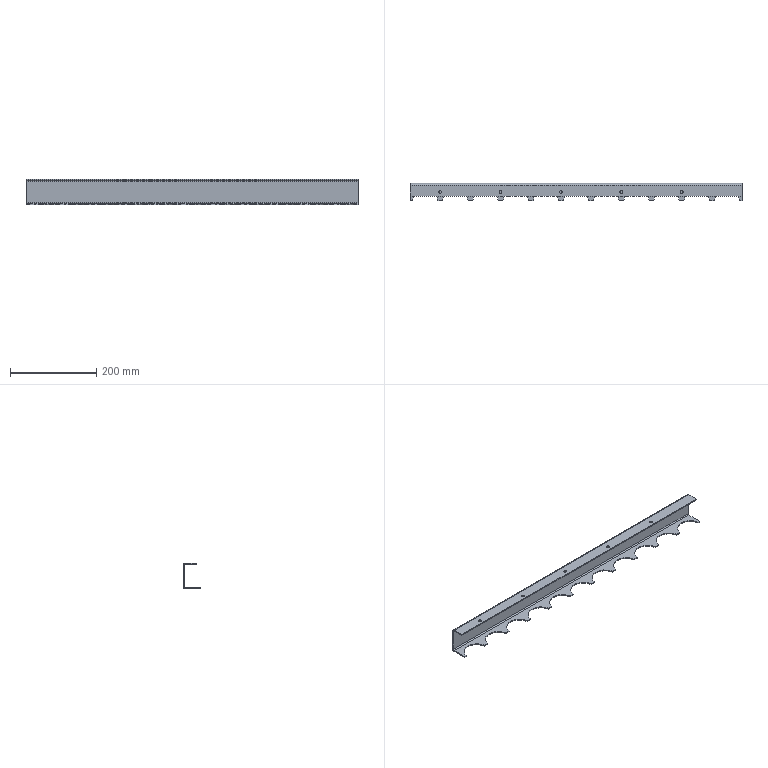Part | STEP file | cc-coverrollers-10 | 1 solid | 41 faces | box 767.8 x 40 x 60 mm | volume 202679 mm3 | plane 21 | cylinder 15 | spline 5 | commonest cylinder face diameters 60 x11 5 x2 10 x2